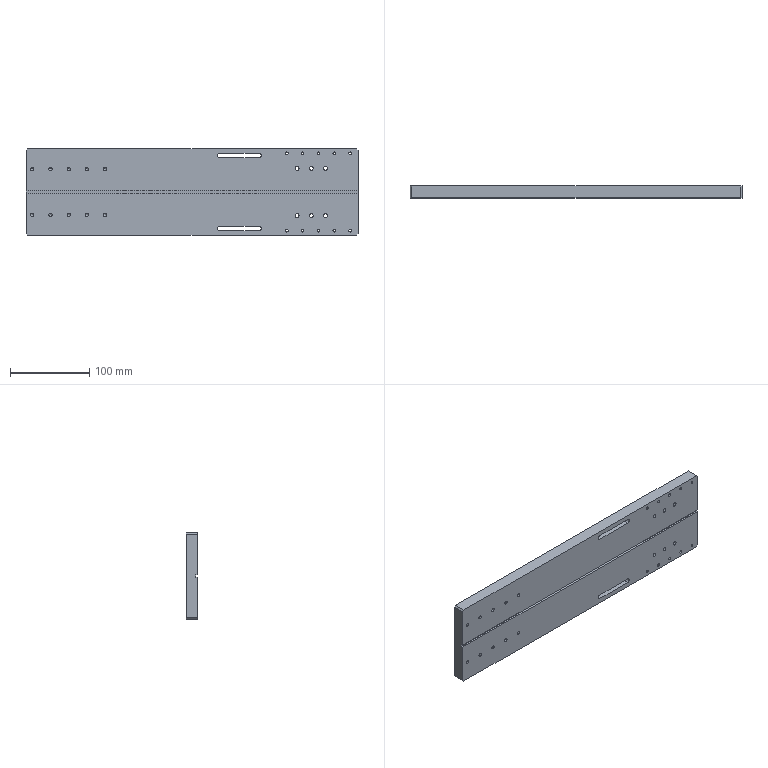Part | STEP file | 11-FG-S00911 | 1 solid | 96 faces | box 420 x 15 x 110 mm | volume 675941 mm3 | cylinder 58 | cone 20 | plane 18 | commonest cylinder face diameters 3.3 x20 4.2 x20 5 x12 5.5 x6